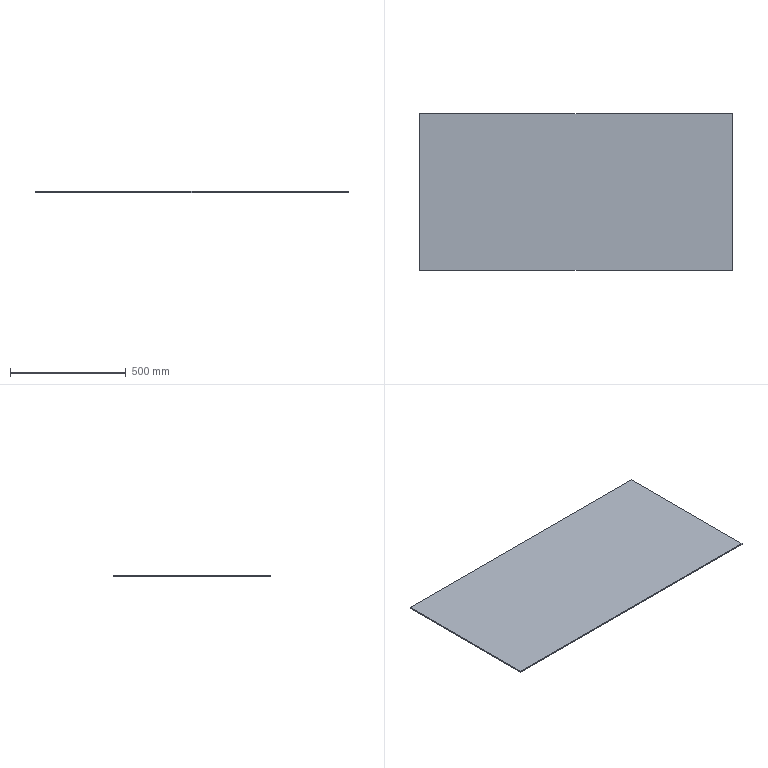Part | SolidWorks | features Extrusion 1, HoleWzd 1 | 1 solid | 6 faces | box 1350 x 676 x 5 mm | volume 4563000 mm3 | plane 6
STEP:
#1=CARTESIAN_POINT('',(675.,-338.,0.));
#2=VERTEX_POINT('',#1);
#3=CARTESIAN_POINT('',(675.,338.,0.));
#4=VERTEX_POINT('',#3);
#5=CARTESIAN_POINT('',(675.,338.,0.));
#6=DIRECTION('',(0.,1.,0.));
#7=VECTOR('',#6,1000.);
#8=LINE('',#5,#7);
#9=EDGE_CURVE('',#2,#4,#8,.T.);
#10=ORIENTED_EDGE('',*,*,#9,.T.);
#11=CARTESIAN_POINT('',(675.,338.,5.));
#12=VERTEX_POINT('',#11);
#13=CARTESIAN_POINT('',(675.,338.,5.));
#14=DIRECTION('',(0.,0.,-1.));
#15=VECTOR('',#14,1000.);
#16=LINE('',#13,#15);
#17=EDGE_CURVE('',#12,#4,#16,.T.);
#18=ORIENTED_EDGE('',*,*,#17,.F.);
#19=CARTESIAN_POINT('',(675.,-338.,5.));
#20=VERTEX_POINT('',#19);
#21=CARTESIAN_POINT('',(675.,338.,5.));
#22=DIRECTION('',(0.,1.,0.));
#23=VECTOR('',#22,1000.);
#24=LINE('',#21,#23);
#25=EDGE_CURVE('',#20,#12,#24,.T.);
#26=ORIENTED_EDGE('',*,*,#25,.F.);
#27=CARTESIAN_POINT('',(675.,-338.,5.));
#28=DIRECTION('',(0.,0.,-1.));
#29=VECTOR('',#28,1000.);
#30=LINE('',#27,#29);
#31=EDGE_CURVE('',#20,#2,#30,.T.);
#32=ORIENTED_EDGE('',*,*,#31,.T.);
#33=EDGE_LOOP('',(#10,#18,#26,#32));
#34=FACE_OUTER_BOUND('',#33,.T.);
#35=CARTESIAN_POINT('',(675.,338.,5.));
#36=DIRECTION('',(-1.,0.,0.));
#37=DIRECTION('',(0.,-1.,0.));
#38=AXIS2_PLACEMENT_3D('',#35,#36,#37);
#39=PLANE('',#38);
#40=ADVANCED_FACE('',(#34),#39,.F.);
#41=CARTESIAN_POINT('',(-675.,338.,0.));
#42=VERTEX_POINT('',#41);
#43=CARTESIAN_POINT('',(-675.,338.,0.));
#44=DIRECTION('',(-1.,0.,0.));
#45=VECTOR('',#44,1000.);
#46=LINE('',#43,#45);
#47=EDGE_CURVE('',#4,#42,#46,.T.);
#48=ORIENTED_EDGE('',*,*,#47,.T.);
#49=CARTESIAN_POINT('',(-675.,338.,5.));
#50=VERTEX_POINT('',#49);
#51=CARTESIAN_POINT('',(-675.,338.,5.));
#52=DIRECTION('',(0.,0.,-1.));
#53=VECTOR('',#52,1000.);
#54=LINE('',#51,#53);
#55=EDGE_CURVE('',#50,#42,#54,.T.);
#56=ORIENTED_EDGE('',*,*,#55,.F.);
#57=CARTESIAN_POINT('',(-675.,338.,5.));
#58=DIRECTION('',(-1.,0.,0.));
#59=VECTOR('',#58,1000.);
#60=LINE('',#57,#59);
#61=EDGE_CURVE('',#12,#50,#60,.T.);
#62=ORIENTED_EDGE('',*,*,#61,.F.);
#63=ORIENTED_EDGE('',*,*,#17,.T.);
#64=EDGE_LOOP('',(#48,#56,#62,#63));
#65=FACE_OUTER_BOUND('',#64,.T.);
#66=CARTESIAN_POINT('',(-675.,338.,5.));
#67=DIRECTION('',(0.,-1.,0.));
#68=DIRECTION('',(0.,0.,-1.));
#69=AXIS2_PLACEMENT_3D('',#66,#67,#68);
#70=PLANE('',#69);
#71=ADVANCED_FACE('',(#65),#70,.F.);
#72=CARTESIAN_POINT('',(-675.,-338.,0.));
#73=VERTEX_POINT('',#72);
#74=CARTESIAN_POINT('',(-675.,338.,0.));
#75=DIRECTION('',(0.,-1.,0.));
#76=VECTOR('',#75,1000.);
#77=LINE('',#74,#76);
#78=EDGE_CURVE('',#42,#73,#77,.T.);
#79=ORIENTED_EDGE('',*,*,#78,.T.);
#80=CARTESIAN_POINT('',(-675.,-338.,5.));
#81=VERTEX_POINT('',#80);
#82=CARTESIAN_POINT('',(-675.,-338.,5.));
#83=DIRECTION('',(0.,0.,-1.));
#84=VECTOR('',#83,1000.);
#85=LINE('',#82,#84);
#86=EDGE_CURVE('',#81,#73,#85,.T.);
#87=ORIENTED_EDGE('',*,*,#86,.F.);
#88=CARTESIAN_POINT('',(-675.,338.,5.));
#89=DIRECTION('',(0.,-1.,0.));
#90=VECTOR('',#89,1000.);
#91=LINE('',#88,#90);
#92=EDGE_CURVE('',#50,#81,#91,.T.);
#93=ORIENTED_EDGE('',*,*,#92,.F.);
#94=ORIENTED_EDGE('',*,*,#55,.T.);
#95=EDGE_LOOP('',(#79,#87,#93,#94));
#96=FACE_OUTER_BOUND('',#95,.T.);
#97=CARTESIAN_POINT('',(-675.,338.,5.));
#98=DIRECTION('',(1.,0.,0.));
#99=DIRECTION('',(0.,0.,-1.));
#100=AXIS2_PLACEMENT_3D('',#97,#98,#99);
#101=PLANE('',#100);
#102=ADVANCED_FACE('',(#96),#101,.F.);
#103=CARTESIAN_POINT('',(-675.,-338.,0.));
#104=DIRECTION('',(1.,0.,0.));
#105=VECTOR('',#104,1000.);
#106=LINE('',#103,#105);
#107=EDGE_CURVE('',#73,#2,#106,.T.);
#108=ORIENTED_EDGE('',*,*,#107,.T.);
#109=ORIENTED_EDGE('',*,*,#31,.F.);
#110=CARTESIAN_POINT('',(-675.,-338.,5.));
#111=DIRECTION('',(1.,0.,0.));
#112=VECTOR('',#111,1000.);
#113=LINE('',#110,#112);
#114=EDGE_CURVE('',#81,#20,#113,.T.);
#115=ORIENTED_EDGE('',*,*,#114,.F.);
#116=ORIENTED_EDGE('',*,*,#86,.T.);
#117=EDGE_LOOP('',(#108,#109,#115,#116));
#118=FACE_OUTER_BOUND('',#117,.T.);
#119=CARTESIAN_POINT('',(-675.,-338.,5.));
#120=DIRECTION('',(0.,1.,0.));
#121=DIRECTION('',(0.,0.,1.));
#122=AXIS2_PLACEMENT_3D('',#119,#120,#121);
#123=PLANE('',#122);
#124=ADVANCED_FACE('',(#118),#123,.F.);
#125=ORIENTED_EDGE('',*,*,#25,.T.);
#126=ORIENTED_EDGE('',*,*,#61,.T.);
#127=ORIENTED_EDGE('',*,*,#92,.T.);
#128=ORIENTED_EDGE('',*,*,#114,.T.);
#129=EDGE_LOOP('',(#125,#126,#127,#128));
#130=FACE_OUTER_BOUND('',#129,.T.);
#131=CARTESIAN_POINT('',(0.,0.,5.));
#132=DIRECTION('',(0.,0.,1.));
#133=DIRECTION('',(1.,0.,0.));
#134=AXIS2_PLACEMENT_3D('',#131,#132,#133);
#135=PLANE('',#134);
#136=ADVANCED_FACE('',(#130),#135,.T.);
#137=ORIENTED_EDGE('',*,*,#9,.F.);
#138=ORIENTED_EDGE('',*,*,#107,.F.);
#139=ORIENTED_EDGE('',*,*,#78,.F.);
#140=ORIENTED_EDGE('',*,*,#47,.F.);
#141=EDGE_LOOP('',(#137,#138,#139,#140));
#142=FACE_OUTER_BOUND('',#141,.T.);
#143=CARTESIAN_POINT('',(0.,0.,0.));
#144=DIRECTION('',(0.,0.,1.));
#145=DIRECTION('',(1.,0.,0.));
#146=AXIS2_PLACEMENT_3D('',#143,#144,#145);
#147=PLANE('',#146);
#148=ADVANCED_FACE('',(#142),#147,.F.);
#149=CLOSED_SHELL('',(#40,#71,#102,#124,#136,#148));
#150=MANIFOLD_SOLID_BREP('',#149);
#151=CARTESIAN_POINT('',(0.,0.,0.));
#152=DIRECTION('',(0.,0.,1.));
#153=DIRECTION('',(1.,0.,0.));
#154=AXIS2_PLACEMENT_3D('',#151,#152,#153);
#155=(LENGTH_UNIT()NAMED_UNIT(*)SI_UNIT(.MILLI.,.METRE.));
#156=UNCERTAINTY_MEASURE_WITH_UNIT(LENGTH_MEASURE(0.00001),#155,'','');
#157=(NAMED_UNIT(*)PLANE_ANGLE_UNIT()SI_UNIT($,.RADIAN.));
#158=(NAMED_UNIT(*)SI_UNIT($,.STERADIAN.)SOLID_ANGLE_UNIT());
#159=(GEOMETRIC_REPRESENTATION_CONTEXT(3)GLOBAL_UNCERTAINTY_ASSIGNED_CONTEXT((#156))GLOBAL_UNIT_ASSIGNED_CONTEXT((#155,#157,#158))REPRESENTATION_CONTEXT('',''));
#160=ADVANCED_BREP_SHAPE_REPRESENTATION('',(#150,#154),#159);